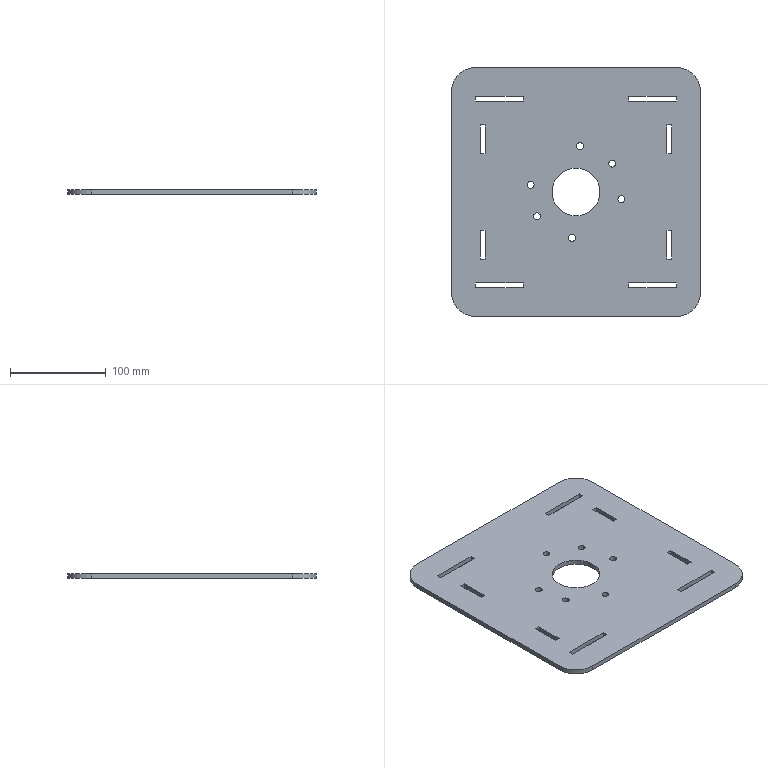Part | SolidWorks | features FlatPattern 1, SMBaseFlange 1, SheetMetal 1 | 1 solid | 56 faces | box 260 x 260 x 5 mm | volume 316279 mm3 | plane 38 | cylinder 18 | commonest cylinder face diameters 7.2 x12 50 x6